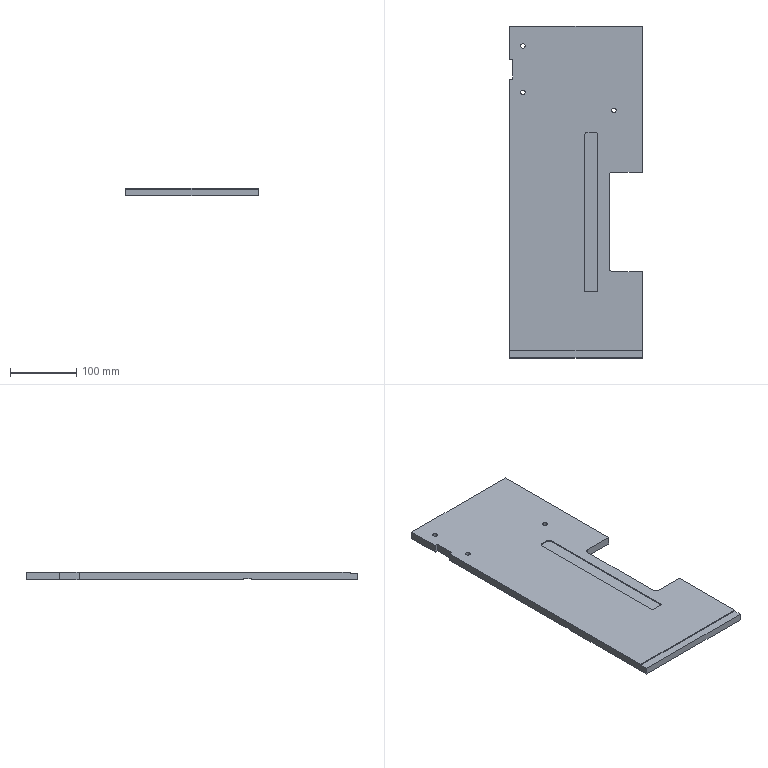Part | SolidWorks | features ICE 6, Fillet 2, Extrusion 1 | 1 solid | 35 faces | box 200 x 500 x 12 mm | volume 1093684 mm3 | plane 25 | cylinder 10 | commonest cylinder face diameters 7 x6 10 x4
STEP:
#1=CARTESIAN_POINT('',(-83.5,220.,-6.));
#2=VERTEX_POINT('',#1);
#3=CARTESIAN_POINT('',(-76.5,220.,-6.));
#4=VERTEX_POINT('',#3);
#5=CARTESIAN_POINT('',(-80.,220.,-6.));
#6=DIRECTION('',(0.,0.,1.));
#7=DIRECTION('',(-1.,0.,0.));
#8=AXIS2_PLACEMENT_3D('',#5,#6,#7);
#9=CIRCLE('',#8,3.5);
#10=EDGE_CURVE('',#2,#4,#9,.T.);
#11=ORIENTED_EDGE('',*,*,#10,.F.);
#12=CARTESIAN_POINT('',(-83.5,220.,6.));
#13=VERTEX_POINT('',#12);
#14=CARTESIAN_POINT('',(-83.5,220.,-6.001));
#15=DIRECTION('',(0.,0.,1.));
#16=VECTOR('',#15,1000.);
#17=LINE('',#14,#16);
#18=EDGE_CURVE('',#2,#13,#17,.T.);
#19=ORIENTED_EDGE('',*,*,#18,.T.);
#20=CARTESIAN_POINT('',(-76.5,220.,6.));
#21=VERTEX_POINT('',#20);
#22=CARTESIAN_POINT('',(-80.,220.,6.));
#23=DIRECTION('',(0.,0.,1.));
#24=DIRECTION('',(1.,0.,0.));
#25=AXIS2_PLACEMENT_3D('',#22,#23,#24);
#26=CIRCLE('',#25,3.5);
#27=EDGE_CURVE('',#13,#21,#26,.T.);
#28=ORIENTED_EDGE('',*,*,#27,.T.);
#29=CARTESIAN_POINT('',(-76.5,220.,-6.001));
#30=DIRECTION('',(0.,0.,1.));
#31=VECTOR('',#30,1000.);
#32=LINE('',#29,#31);
#33=EDGE_CURVE('',#4,#21,#32,.T.);
#34=ORIENTED_EDGE('',*,*,#33,.F.);
#35=EDGE_LOOP('',(#11,#19,#28,#34));
#36=FACE_OUTER_BOUND('',#35,.T.);
#37=CARTESIAN_POINT('',(-80.,220.,-6.001));
#38=DIRECTION('',(0.,0.,1.));
#39=DIRECTION('',(1.,0.,0.));
#40=AXIS2_PLACEMENT_3D('',#37,#38,#39);
#41=CYLINDRICAL_SURFACE('',#40,3.5);
#42=ADVANCED_FACE('',(#36),#41,.F.);
#43=CARTESIAN_POINT('',(-83.5,150.,-6.));
#44=VERTEX_POINT('',#43);
#45=CARTESIAN_POINT('',(-76.5,150.,-6.));
#46=VERTEX_POINT('',#45);
#47=CARTESIAN_POINT('',(-80.,150.,-6.));
#48=DIRECTION('',(0.,0.,1.));
#49=DIRECTION('',(-1.,0.,0.));
#50=AXIS2_PLACEMENT_3D('',#47,#48,#49);
#51=CIRCLE('',#50,3.5);
#52=EDGE_CURVE('',#44,#46,#51,.T.);
#53=ORIENTED_EDGE('',*,*,#52,.F.);
#54=CARTESIAN_POINT('',(-83.5,150.,6.));
#55=VERTEX_POINT('',#54);
#56=CARTESIAN_POINT('',(-83.5,150.,-6.001));
#57=DIRECTION('',(0.,0.,1.));
#58=VECTOR('',#57,1000.);
#59=LINE('',#56,#58);
#60=EDGE_CURVE('',#44,#55,#59,.T.);
#61=ORIENTED_EDGE('',*,*,#60,.T.);
#62=CARTESIAN_POINT('',(-76.5,150.,6.));
#63=VERTEX_POINT('',#62);
#64=CARTESIAN_POINT('',(-80.,150.,6.));
#65=DIRECTION('',(0.,0.,1.));
#66=DIRECTION('',(1.,0.,0.));
#67=AXIS2_PLACEMENT_3D('',#64,#65,#66);
#68=CIRCLE('',#67,3.5);
#69=EDGE_CURVE('',#55,#63,#68,.T.);
#70=ORIENTED_EDGE('',*,*,#69,.T.);
#71=CARTESIAN_POINT('',(-76.5,150.,-6.001));
#72=DIRECTION('',(0.,0.,1.));
#73=VECTOR('',#72,1000.);
#74=LINE('',#71,#73);
#75=EDGE_CURVE('',#46,#63,#74,.T.);
#76=ORIENTED_EDGE('',*,*,#75,.F.);
#77=EDGE_LOOP('',(#53,#61,#70,#76));
#78=FACE_OUTER_BOUND('',#77,.T.);
#79=CARTESIAN_POINT('',(-80.,150.,-6.001));
#80=DIRECTION('',(0.,0.,1.));
#81=DIRECTION('',(1.,0.,0.));
#82=AXIS2_PLACEMENT_3D('',#79,#80,#81);
#83=CYLINDRICAL_SURFACE('',#82,3.5);
#84=ADVANCED_FACE('',(#78),#83,.F.);
#85=CARTESIAN_POINT('',(53.5,123.,-6.));
#86=VERTEX_POINT('',#85);
#87=CARTESIAN_POINT('',(60.5,123.,-6.));
#88=VERTEX_POINT('',#87);
#89=CARTESIAN_POINT('',(57.,123.,-6.));
#90=DIRECTION('',(0.,0.,1.));
#91=DIRECTION('',(-1.,0.,0.));
#92=AXIS2_PLACEMENT_3D('',#89,#90,#91);
#93=CIRCLE('',#92,3.5);
#94=EDGE_CURVE('',#86,#88,#93,.T.);
#95=ORIENTED_EDGE('',*,*,#94,.F.);
#96=CARTESIAN_POINT('',(53.5,123.,6.));
#97=VERTEX_POINT('',#96);
#98=CARTESIAN_POINT('',(53.5,123.,-6.001));
#99=DIRECTION('',(0.,0.,1.));
#100=VECTOR('',#99,1000.);
#101=LINE('',#98,#100);
#102=EDGE_CURVE('',#86,#97,#101,.T.);
#103=ORIENTED_EDGE('',*,*,#102,.T.);
#104=CARTESIAN_POINT('',(60.5,123.,6.));
#105=VERTEX_POINT('',#104);
#106=CARTESIAN_POINT('',(57.,123.,6.));
#107=DIRECTION('',(0.,0.,1.));
#108=DIRECTION('',(1.,0.,0.));
#109=AXIS2_PLACEMENT_3D('',#106,#107,#108);
#110=CIRCLE('',#109,3.5);
#111=EDGE_CURVE('',#97,#105,#110,.T.);
#112=ORIENTED_EDGE('',*,*,#111,.T.);
#113=CARTESIAN_POINT('',(60.5,123.,-6.001));
#114=DIRECTION('',(0.,0.,1.));
#115=VECTOR('',#114,1000.);
#116=LINE('',#113,#115);
#117=EDGE_CURVE('',#88,#105,#116,.T.);
#118=ORIENTED_EDGE('',*,*,#117,.F.);
#119=EDGE_LOOP('',(#95,#103,#112,#118));
#120=FACE_OUTER_BOUND('',#119,.T.);
#121=CARTESIAN_POINT('',(57.,123.,-6.001));
#122=DIRECTION('',(0.,0.,1.));
#123=DIRECTION('',(1.,0.,0.));
#124=AXIS2_PLACEMENT_3D('',#121,#122,#123);
#125=CYLINDRICAL_SURFACE('',#124,3.5);
#126=ADVANCED_FACE('',(#120),#125,.F.);
#127=CARTESIAN_POINT('',(100.,30.,6.));
#128=VERTEX_POINT('',#127);
#129=CARTESIAN_POINT('',(100.,250.,6.));
#130=VERTEX_POINT('',#129);
#131=CARTESIAN_POINT('',(100.,-250.,6.));
#132=DIRECTION('',(0.,1.,0.));
#133=VECTOR('',#132,1000.);
#134=LINE('',#131,#133);
#135=EDGE_CURVE('',#128,#130,#134,.T.);
#136=ORIENTED_EDGE('',*,*,#135,.F.);
#137=CARTESIAN_POINT('',(100.,30.,-6.));
#138=VERTEX_POINT('',#137);
#139=CARTESIAN_POINT('',(100.,30.,6.001));
#140=DIRECTION('',(0.,0.,-1.));
#141=VECTOR('',#140,1000.);
#142=LINE('',#139,#141);
#143=EDGE_CURVE('',#128,#138,#142,.T.);
#144=ORIENTED_EDGE('',*,*,#143,.T.);
#145=CARTESIAN_POINT('',(100.,250.,-6.));
#146=VERTEX_POINT('',#145);
#147=CARTESIAN_POINT('',(100.,-250.,-6.));
#148=DIRECTION('',(0.,1.,0.));
#149=VECTOR('',#148,1000.);
#150=LINE('',#147,#149);
#151=EDGE_CURVE('',#138,#146,#150,.T.);
#152=ORIENTED_EDGE('',*,*,#151,.T.);
#153=CARTESIAN_POINT('',(100.,250.,6.));
#154=DIRECTION('',(0.,0.,-1.));
#155=VECTOR('',#154,1000.);
#156=LINE('',#153,#155);
#157=EDGE_CURVE('',#130,#146,#156,.T.);
#158=ORIENTED_EDGE('',*,*,#157,.F.);
#159=EDGE_LOOP('',(#136,#144,#152,#158));
#160=FACE_OUTER_BOUND('',#159,.T.);
#161=CARTESIAN_POINT('',(100.,-250.,6.));
#162=DIRECTION('',(-1.,0.,0.));
#163=DIRECTION('',(0.,0.,1.));
#164=AXIS2_PLACEMENT_3D('',#161,#162,#163);
#165=PLANE('',#164);
#166=ADVANCED_FACE('',(#160),#165,.F.);
#167=CARTESIAN_POINT('',(-100.,170.,6.));
#168=VERTEX_POINT('',#167);
#169=CARTESIAN_POINT('',(-100.,-238.,6.));
#170=VERTEX_POINT('',#169);
#171=CARTESIAN_POINT('',(-100.,-250.,6.));
#172=DIRECTION('',(0.,-1.,0.));
#173=VECTOR('',#172,1000.);
#174=LINE('',#171,#173);
#175=EDGE_CURVE('',#168,#170,#174,.T.);
#176=ORIENTED_EDGE('',*,*,#175,.T.);
#177=CARTESIAN_POINT('',(100.,-238.,6.));
#178=VERTEX_POINT('',#177);
#179=CARTESIAN_POINT('',(-100.,-238.,6.));
#180=DIRECTION('',(-1.,0.,0.));
#181=VECTOR('',#180,1000.);
#182=LINE('',#179,#181);
#183=EDGE_CURVE('',#178,#170,#182,.T.);
#184=ORIENTED_EDGE('',*,*,#183,.F.);
#185=CARTESIAN_POINT('',(100.,-120.,6.));
#186=VERTEX_POINT('',#185);
#187=CARTESIAN_POINT('',(100.,-250.,6.));
#188=DIRECTION('',(0.,1.,0.));
#189=VECTOR('',#188,1000.);
#190=LINE('',#187,#189);
#191=EDGE_CURVE('',#178,#186,#190,.T.);
#192=ORIENTED_EDGE('',*,*,#191,.T.);
#193=CARTESIAN_POINT('',(55.,-120.,6.));
#194=VERTEX_POINT('',#193);
#195=CARTESIAN_POINT('',(100.,-120.,6.));
#196=DIRECTION('',(1.,0.,0.));
#197=VECTOR('',#196,1000.);
#198=LINE('',#195,#197);
#199=EDGE_CURVE('',#194,#186,#198,.T.);
#200=ORIENTED_EDGE('',*,*,#199,.F.);
#201=CARTESIAN_POINT('',(50.,-115.,6.));
#202=VERTEX_POINT('',#201);
#203=CARTESIAN_POINT('',(55.,-115.,6.));
#204=DIRECTION('',(0.,0.,-1.));
#205=DIRECTION('',(-1.,0.,0.));
#206=AXIS2_PLACEMENT_3D('',#203,#204,#205);
#207=CIRCLE('',#206,5.);
#208=EDGE_CURVE('',#194,#202,#207,.T.);
#209=ORIENTED_EDGE('',*,*,#208,.T.);
#210=CARTESIAN_POINT('',(50.,25.,6.));
#211=VERTEX_POINT('',#210);
#212=CARTESIAN_POINT('',(50.,-120.,6.));
#213=DIRECTION('',(0.,-1.,0.));
#214=VECTOR('',#213,1000.);
#215=LINE('',#212,#214);
#216=EDGE_CURVE('',#211,#202,#215,.T.);
#217=ORIENTED_EDGE('',*,*,#216,.F.);
#218=CARTESIAN_POINT('',(55.,30.,6.));
#219=VERTEX_POINT('',#218);
#220=CARTESIAN_POINT('',(55.,25.,6.));
#221=DIRECTION('',(0.,0.,-1.));
#222=DIRECTION('',(-1.,0.,0.));
#223=AXIS2_PLACEMENT_3D('',#220,#221,#222);
#224=CIRCLE('',#223,5.);
#225=EDGE_CURVE('',#211,#219,#224,.T.);
#226=ORIENTED_EDGE('',*,*,#225,.T.);
#227=CARTESIAN_POINT('',(100.,30.,6.));
#228=DIRECTION('',(-1.,0.,0.));
#229=VECTOR('',#228,1000.);
#230=LINE('',#227,#229);
#231=EDGE_CURVE('',#128,#219,#230,.T.);
#232=ORIENTED_EDGE('',*,*,#231,.F.);
#233=ORIENTED_EDGE('',*,*,#135,.T.);
#234=CARTESIAN_POINT('',(-100.,250.,6.));
#235=VERTEX_POINT('',#234);
#236=CARTESIAN_POINT('',(-100.,250.,6.));
#237=DIRECTION('',(-1.,0.,0.));
#238=VECTOR('',#237,1000.);
#239=LINE('',#236,#238);
#240=EDGE_CURVE('',#130,#235,#239,.T.);
#241=ORIENTED_EDGE('',*,*,#240,.T.);
#242=CARTESIAN_POINT('',(-100.,200.,6.));
#243=VERTEX_POINT('',#242);
#244=CARTESIAN_POINT('',(-100.,-250.,6.));
#245=DIRECTION('',(0.,-1.,0.));
#246=VECTOR('',#245,1000.);
#247=LINE('',#244,#246);
#248=EDGE_CURVE('',#235,#243,#247,.T.);
#249=ORIENTED_EDGE('',*,*,#248,.T.);
#250=CARTESIAN_POINT('',(-95.,200.,6.));
#251=VERTEX_POINT('',#250);
#252=CARTESIAN_POINT('',(-95.,200.,6.));
#253=DIRECTION('',(-1.,0.,0.));
#254=VECTOR('',#253,1000.);
#255=LINE('',#252,#254);
#256=EDGE_CURVE('',#251,#243,#255,.T.);
#257=ORIENTED_EDGE('',*,*,#256,.F.);
#258=CARTESIAN_POINT('',(-95.,170.,6.));
#259=VERTEX_POINT('',#258);
#260=CARTESIAN_POINT('',(-95.,170.,6.));
#261=DIRECTION('',(0.,1.,0.));
#262=VECTOR('',#261,1000.);
#263=LINE('',#260,#262);
#264=EDGE_CURVE('',#259,#251,#263,.T.);
#265=ORIENTED_EDGE('',*,*,#264,.F.);
#266=CARTESIAN_POINT('',(-100.,170.,6.));
#267=DIRECTION('',(1.,0.,0.));
#268=VECTOR('',#267,1000.);
#269=LINE('',#266,#268);
#270=EDGE_CURVE('',#168,#259,#269,.T.);
#271=ORIENTED_EDGE('',*,*,#270,.F.);
#272=EDGE_LOOP('',(#176,#184,#192,#200,#209,#217,#226,#232,#233,#241,#249,#257,#265,#271));
#273=FACE_OUTER_BOUND('',#272,.T.);
#274=CARTESIAN_POINT('',(57.,123.,6.));
#275=DIRECTION('',(0.,0.,1.));
#276=DIRECTION('',(1.,0.,0.));
#277=AXIS2_PLACEMENT_3D('',#274,#275,#276);
#278=CIRCLE('',#277,3.5);
#279=EDGE_CURVE('',#105,#97,#278,.T.);
#280=ORIENTED_EDGE('',*,*,#279,.F.);
#281=ORIENTED_EDGE('',*,*,#111,.F.);
#282=EDGE_LOOP('',(#280,#281));
#283=FACE_BOUND('',#282,.T.);
#284=CARTESIAN_POINT('',(-80.,150.,6.));
#285=DIRECTION('',(0.,0.,1.));
#286=DIRECTION('',(1.,0.,0.));
#287=AXIS2_PLACEMENT_3D('',#284,#285,#286);
#288=CIRCLE('',#287,3.5);
#289=EDGE_CURVE('',#63,#55,#288,.T.);
#290=ORIENTED_EDGE('',*,*,#289,.F.);
#291=ORIENTED_EDGE('',*,*,#69,.F.);
#292=EDGE_LOOP('',(#290,#291));
#293=FACE_BOUND('',#292,.T.);
#294=CARTESIAN_POINT('',(-80.,220.,6.));
#295=DIRECTION('',(0.,0.,1.));
#296=DIRECTION('',(1.,0.,0.));
#297=AXIS2_PLACEMENT_3D('',#294,#295,#296);
#298=CIRCLE('',#297,3.5);
#299=EDGE_CURVE('',#21,#13,#298,.T.);
#300=ORIENTED_EDGE('',*,*,#299,.F.);
#301=ORIENTED_EDGE('',*,*,#27,.F.);
#302=EDGE_LOOP('',(#300,#301));
#303=FACE_BOUND('',#302,.T.);
#304=CARTESIAN_POINT('',(18.,90.,6.));
#305=VERTEX_POINT('',#304);
#306=CARTESIAN_POINT('',(28.,90.,6.));
#307=VERTEX_POINT('',#306);
#308=CARTESIAN_POINT('',(33.,90.,6.));
#309=DIRECTION('',(1.,0.,0.));
#310=VECTOR('',#309,1000.);
#311=LINE('',#308,#310);
#312=EDGE_CURVE('',#305,#307,#311,.T.);
#313=ORIENTED_EDGE('',*,*,#312,.T.);
#314=CARTESIAN_POINT('',(33.,85.,6.));
#315=VERTEX_POINT('',#314);
#316=CARTESIAN_POINT('',(28.,85.,6.));
#317=DIRECTION('',(0.,0.,-1.));
#318=DIRECTION('',(-1.,0.,0.));
#319=AXIS2_PLACEMENT_3D('',#316,#317,#318);
#320=CIRCLE('',#319,5.);
#321=EDGE_CURVE('',#307,#315,#320,.T.);
#322=ORIENTED_EDGE('',*,*,#321,.T.);
#323=CARTESIAN_POINT('',(33.,-150.,6.));
#324=VERTEX_POINT('',#323);
#325=CARTESIAN_POINT('',(33.,-150.,6.));
#326=DIRECTION('',(0.,-1.,0.));
#327=VECTOR('',#326,1000.);
#328=LINE('',#325,#327);
#329=EDGE_CURVE('',#315,#324,#328,.T.);
#330=ORIENTED_EDGE('',*,*,#329,.T.);
#331=CARTESIAN_POINT('',(13.,-150.,6.));
#332=VERTEX_POINT('',#331);
#333=CARTESIAN_POINT('',(33.,-150.,6.));
#334=DIRECTION('',(-1.,0.,0.));
#335=VECTOR('',#334,1000.);
#336=LINE('',#333,#335);
#337=EDGE_CURVE('',#324,#332,#336,.T.);
#338=ORIENTED_EDGE('',*,*,#337,.T.);
#339=CARTESIAN_POINT('',(13.,85.,6.));
#340=VERTEX_POINT('',#339);
#341=CARTESIAN_POINT('',(13.,-150.,6.));
#342=DIRECTION('',(0.,1.,0.));
#343=VECTOR('',#342,1000.);
#344=LINE('',#341,#343);
#345=EDGE_CURVE('',#332,#340,#344,.T.);
#346=ORIENTED_EDGE('',*,*,#345,.T.);
#347=CARTESIAN_POINT('',(18.,85.,6.));
#348=DIRECTION('',(0.,0.,-1.));
#349=DIRECTION('',(-1.,0.,0.));
#350=AXIS2_PLACEMENT_3D('',#347,#348,#349);
#351=CIRCLE('',#350,5.);
#352=EDGE_CURVE('',#340,#305,#351,.T.);
#353=ORIENTED_EDGE('',*,*,#352,.T.);
#354=EDGE_LOOP('',(#313,#322,#330,#338,#346,#353));
#355=FACE_BOUND('',#354,.T.);
#356=CARTESIAN_POINT('',(0.,0.,6.));
#357=DIRECTION('',(0.,0.,-1.));
#358=DIRECTION('',(-1.,0.,0.));
#359=AXIS2_PLACEMENT_3D('',#356,#357,#358);
#360=PLANE('',#359);
#361=ADVANCED_FACE('',(#273,#283,#293,#303,#355),#360,.F.);
#362=CARTESIAN_POINT('',(-100.,-238.,4.5));
#363=VERTEX_POINT('',#362);
#364=CARTESIAN_POINT('',(-100.,-250.,4.5));
#365=VERTEX_POINT('',#364);
#366=CARTESIAN_POINT('',(-100.,-250.,4.5));
#367=DIRECTION('',(0.,-1.,0.));
#368=VECTOR('',#367,1000.);
#369=LINE('',#366,#368);
#370=EDGE_CURVE('',#363,#365,#369,.T.);
#371=ORIENTED_EDGE('',*,*,#370,.F.);
#372=CARTESIAN_POINT('',(-100.,-238.,4.5));
#373=DIRECTION('',(0.,0.,1.));
#374=VECTOR('',#373,1000.);
#375=LINE('',#372,#374);
#376=EDGE_CURVE('',#363,#170,#375,.T.);
#377=ORIENTED_EDGE('',*,*,#376,.T.);
#378=ORIENTED_EDGE('',*,*,#175,.F.);
#379=CARTESIAN_POINT('',(-100.,170.,-6.));
#380=VERTEX_POINT('',#379);
#381=CARTESIAN_POINT('',(-100.,170.,-6.001));
#382=DIRECTION('',(0.,0.,1.));
#383=VECTOR('',#382,1000.);
#384=LINE('',#381,#383);
#385=EDGE_CURVE('',#380,#168,#384,.T.);
#386=ORIENTED_EDGE('',*,*,#385,.F.);
#387=CARTESIAN_POINT('',(-100.,-78.,-6.));
#388=VERTEX_POINT('',#387);
#389=CARTESIAN_POINT('',(-100.,-250.,-6.));
#390=DIRECTION('',(0.,-1.,0.));
#391=VECTOR('',#390,1000.);
#392=LINE('',#389,#391);
#393=EDGE_CURVE('',#380,#388,#392,.T.);
#394=ORIENTED_EDGE('',*,*,#393,.T.);
#395=CARTESIAN_POINT('',(-100.,-78.,-4.5));
#396=VERTEX_POINT('',#395);
#397=CARTESIAN_POINT('',(-100.,-78.,-4.5));
#398=DIRECTION('',(0.,0.,-1.));
#399=VECTOR('',#398,1000.);
#400=LINE('',#397,#399);
#401=EDGE_CURVE('',#396,#388,#400,.T.);
#402=ORIENTED_EDGE('',*,*,#401,.F.);
#403=CARTESIAN_POINT('',(-100.,-89.,-4.5));
#404=VERTEX_POINT('',#403);
#405=CARTESIAN_POINT('',(-100.,-89.,-4.5));
#406=DIRECTION('',(0.,-1.,0.));
#407=VECTOR('',#406,1000.);
#408=LINE('',#405,#407);
#409=EDGE_CURVE('',#396,#404,#408,.T.);
#410=ORIENTED_EDGE('',*,*,#409,.T.);
#411=CARTESIAN_POINT('',(-100.,-89.,-6.));
#412=VERTEX_POINT('',#411);
#413=CARTESIAN_POINT('',(-100.,-89.,-4.5));
#414=DIRECTION('',(0.,0.,-1.));
#415=VECTOR('',#414,1000.);
#416=LINE('',#413,#415);
#417=EDGE_CURVE('',#404,#412,#416,.T.);
#418=ORIENTED_EDGE('',*,*,#417,.T.);
#419=CARTESIAN_POINT('',(-100.,-250.,-6.));
#420=VERTEX_POINT('',#419);
#421=CARTESIAN_POINT('',(-100.,-250.,-6.));
#422=DIRECTION('',(0.,-1.,0.));
#423=VECTOR('',#422,1000.);
#424=LINE('',#421,#423);
#425=EDGE_CURVE('',#412,#420,#424,.T.);
#426=ORIENTED_EDGE('',*,*,#425,.T.);
#427=CARTESIAN_POINT('',(-100.,-250.,6.));
#428=DIRECTION('',(0.,0.,-1.));
#429=VECTOR('',#428,1000.);
#430=LINE('',#427,#429);
#431=EDGE_CURVE('',#365,#420,#430,.T.);
#432=ORIENTED_EDGE('',*,*,#431,.F.);
#433=EDGE_LOOP('',(#371,#377,#378,#386,#394,#402,#410,#418,#426,#432));
#434=FACE_OUTER_BOUND('',#433,.T.);
#435=CARTESIAN_POINT('',(-100.,-250.,6.));
#436=DIRECTION('',(1.,0.,0.));
#437=DIRECTION('',(0.,0.,-1.));
#438=AXIS2_PLACEMENT_3D('',#435,#436,#437);
#439=PLANE('',#438);
#440=ADVANCED_FACE('',(#434),#439,.F.);
#441=ORIENTED_EDGE('',*,*,#191,.F.);
#442=CARTESIAN_POINT('',(100.,-238.,4.5));
#443=VERTEX_POINT('',#442);
#444=CARTESIAN_POINT('',(100.,-238.,4.5));
#445=DIRECTION('',(0.,0.,1.));
#446=VECTOR('',#445,1000.);
#447=LINE('',#444,#446);
#448=EDGE_CURVE('',#443,#178,#447,.T.);
#449=ORIENTED_EDGE('',*,*,#448,.F.);
#450=CARTESIAN_POINT('',(100.,-250.,4.5));
#451=VERTEX_POINT('',#450);
#452=CARTESIAN_POINT('',(100.,-250.,4.5));
#453=DIRECTION('',(0.,1.,0.));
#454=VECTOR('',#453,1000.);
#455=LINE('',#452,#454);
#456=EDGE_CURVE('',#451,#443,#455,.T.);
#457=ORIENTED_EDGE('',*,*,#456,.F.);
#458=CARTESIAN_POINT('',(100.,-250.,-6.));
#459=VERTEX_POINT('',#458);
#460=CARTESIAN_POINT('',(100.,-250.,6.));
#461=DIRECTION('',(0.,0.,-1.));
#462=VECTOR('',#461,1000.);
#463=LINE('',#460,#462);
#464=EDGE_CURVE('',#451,#459,#463,.T.);
#465=ORIENTED_EDGE('',*,*,#464,.T.);
#466=CARTESIAN_POINT('',(100.,-120.,-6.));
#467=VERTEX_POINT('',#466);
#468=CARTESIAN_POINT('',(100.,-250.,-6.));
#469=DIRECTION('',(0.,1.,0.));
#470=VECTOR('',#469,1000.);
#471=LINE('',#468,#470);
#472=EDGE_CURVE('',#459,#467,#471,.T.);
#473=ORIENTED_EDGE('',*,*,#472,.T.);
#474=CARTESIAN_POINT('',(100.,-120.,6.001));
#475=DIRECTION('',(0.,0.,-1.));
#476=VECTOR('',#475,1000.);
#477=LINE('',#474,#476);
#478=EDGE_CURVE('',#186,#467,#477,.T.);
#479=ORIENTED_EDGE('',*,*,#478,.F.);
#480=EDGE_LOOP('',(#441,#449,#457,#465,#473,#479));
#481=FACE_OUTER_BOUND('',#480,.T.);
#482=CARTESIAN_POINT('',(100.,-250.,6.));
#483=DIRECTION('',(-1.,0.,0.));
#484=DIRECTION('',(0.,0.,1.));
#485=AXIS2_PLACEMENT_3D('',#482,#483,#484);
#486=PLANE('',#485);
#487=ADVANCED_FACE('',(#481),#486,.F.);
#488=CARTESIAN_POINT('',(-100.,250.,-6.));
#489=VERTEX_POINT('',#488);
#490=CARTESIAN_POINT('',(-100.,200.,-6.));
#491=VERTEX_POINT('',#490);
#492=CARTESIAN_POINT('',(-100.,-250.,-6.));
#493=DIRECTION('',(0.,-1.,0.));
#494=VECTOR('',#493,1000.);
#495=LINE('',#492,#494);
#496=EDGE_CURVE('',#489,#491,#495,.T.);
#497=ORIENTED_EDGE('',*,*,#496,.T.);
#498=CARTESIAN_POINT('',(-100.,200.,-6.001));
#499=DIRECTION('',(0.,0.,1.));
#500=VECTOR('',#499,1000.);
#501=LINE('',#498,#500);
#502=EDGE_CURVE('',#491,#243,#501,.T.);
#503=ORIENTED_EDGE('',*,*,#502,.T.);
#504=ORIENTED_EDGE('',*,*,#248,.F.);
#505=CARTESIAN_POINT('',(-100.,250.,6.));
#506=DIRECTION('',(0.,0.,-1.));
#507=VECTOR('',#506,1000.);
#508=LINE('',#505,#507);
#509=EDGE_CURVE('',#235,#489,#508,.T.);
#510=ORIENTED_EDGE('',*,*,#509,.T.);
#511=EDGE_LOOP('',(#497,#503,#504,#510));
#512=FACE_OUTER_BOUND('',#511,.T.);
#513=CARTESIAN_POINT('',(-100.,-250.,6.));
#514=DIRECTION('',(1.,0.,0.));
#515=DIRECTION('',(0.,0.,-1.));
#516=AXIS2_PLACEMENT_3D('',#513,#514,#515);
#517=PLANE('',#516);
#518=ADVANCED_FACE('',(#512),#517,.F.);
#519=CARTESIAN_POINT('',(50.,-115.,-6.));
#520=VERTEX_POINT('',#519);
#521=CARTESIAN_POINT('',(50.,-89.,-6.));
#522=VERTEX_POINT('',#521);
#523=CARTESIAN_POINT('',(50.,-120.,-6.));
#524=DIRECTION('',(0.,1.,0.));
#525=VECTOR('',#524,1000.);
#526=LINE('',#523,#525);
#527=EDGE_CURVE('',#520,#522,#526,.T.);
#528=ORIENTED_EDGE('',*,*,#527,.F.);
#529=CARTESIAN_POINT('',(55.,-120.,-6.));
#530=VERTEX_POINT('',#529);
#531=CARTESIAN_POINT('',(55.,-115.,-6.));
#532=DIRECTION('',(0.,0.,1.));
#533=DIRECTION('',(-1.,0.,0.));
#534=AXIS2_PLACEMENT_3D('',#531,#532,#533);
#535=CIRCLE('',#534,5.);
#536=EDGE_CURVE('',#520,#530,#535,.T.);
#537=ORIENTED_EDGE('',*,*,#536,.T.);
#538=CARTESIAN_POINT('',(100.,-120.,-6.));
#539=DIRECTION('',(-1.,0.,0.));
#540=VECTOR('',#539,1000.);
#541=LINE('',#538,#540);
#542=EDGE_CURVE('',#467,#530,#541,.T.);
#543=ORIENTED_EDGE('',*,*,#542,.F.);
#544=ORIENTED_EDGE('',*,*,#472,.F.);
#545=CARTESIAN_POINT('',(-100.,-250.,-6.));
#546=DIRECTION('',(1.,0.,0.));
#547=VECTOR('',#546,1000.);
#548=LINE('',#545,#547);
#549=EDGE_CURVE('',#420,#459,#548,.T.);
#550=ORIENTED_EDGE('',*,*,#549,.F.);
#551=ORIENTED_EDGE('',*,*,#425,.F.);
#552=CARTESIAN_POINT('',(-100.,-89.,-6.));
#553=DIRECTION('',(1.,0.,0.));
#554=VECTOR('',#553,1000.);
#555=LINE('',#552,#554);
#556=EDGE_CURVE('',#412,#522,#555,.T.);
#557=ORIENTED_EDGE('',*,*,#556,.T.);
#558=EDGE_LOOP('',(#528,#537,#543,#544,#550,#551,#557));
#559=FACE_OUTER_BOUND('',#558,.T.);
#560=CARTESIAN_POINT('',(0.,0.,-6.));
#561=DIRECTION('',(0.,0.,-1.));
#562=DIRECTION('',(-1.,0.,0.));
#563=AXIS2_PLACEMENT_3D('',#560,#561,#562);
#564=PLANE('',#563);
#565=ADVANCED_FACE('',(#559),#564,.T.);
#566=CARTESIAN_POINT('',(55.,30.,-6.));
#567=VERTEX_POINT('',#566);
#568=CARTESIAN_POINT('',(100.,30.,-6.));
#569=DIRECTION('',(1.,0.,0.));
#570=VECTOR('',#569,1000.);
#571=LINE('',#568,#570);
#572=EDGE_CURVE('',#567,#138,#571,.T.);
#573=ORIENTED_EDGE('',*,*,#572,.F.);
#574=CARTESIAN_POINT('',(50.,25.,-6.));
#575=VERTEX_POINT('',#574);
#576=CARTESIAN_POINT('',(55.,25.,-6.));
#577=DIRECTION('',(0.,0.,1.));
#578=DIRECTION('',(-1.,0.,0.));
#579=AXIS2_PLACEMENT_3D('',#576,#577,#578);
#580=CIRCLE('',#579,5.);
#581=EDGE_CURVE('',#567,#575,#580,.T.);
#582=ORIENTED_EDGE('',*,*,#581,.T.);
#583=CARTESIAN_POINT('',(50.,-78.,-6.));
#584=VERTEX_POINT('',#583);
#585=CARTESIAN_POINT('',(50.,-120.,-6.));
#586=DIRECTION('',(0.,1.,0.));
#587=VECTOR('',#586,1000.);
#588=LINE('',#585,#587);
#589=EDGE_CURVE('',#584,#575,#588,.T.);
#590=ORIENTED_EDGE('',*,*,#589,.F.);
#591=CARTESIAN_POINT('',(-100.,-78.,-6.));
#592=DIRECTION('',(-1.,0.,0.));
#593=VECTOR('',#592,1000.);
#594=LINE('',#591,#593);
#595=EDGE_CURVE('',#584,#388,#594,.T.);
#596=ORIENTED_EDGE('',*,*,#595,.T.);
#597=ORIENTED_EDGE('',*,*,#393,.F.);
#598=CARTESIAN_POINT('',(-95.,170.,-6.));
#599=VERTEX_POINT('',#598);
#600=CARTESIAN_POINT('',(-100.,170.,-6.));
#601=DIRECTION('',(1.,0.,0.));
#602=VECTOR('',#601,1000.);
#603=LINE('',#600,#602);
#604=EDGE_CURVE('',#380,#599,#603,.T.);
#605=ORIENTED_EDGE('',*,*,#604,.T.);
#606=CARTESIAN_POINT('',(-95.,200.,-6.));
#607=VERTEX_POINT('',#606);
#608=CARTESIAN_POINT('',(-95.,170.,-6.));
#609=DIRECTION('',(0.,1.,0.));
#610=VECTOR('',#609,1000.);
#611=LINE('',#608,#610);
#612=EDGE_CURVE('',#599,#607,#611,.T.);
#613=ORIENTED_EDGE('',*,*,#612,.T.);
#614=CARTESIAN_POINT('',(-95.,200.,-6.));
#615=DIRECTION('',(-1.,0.,0.));
#616=VECTOR('',#615,1000.);
#617=LINE('',#614,#616);
#618=EDGE_CURVE('',#607,#491,#617,.T.);
#619=ORIENTED_EDGE('',*,*,#618,.T.);
#620=ORIENTED_EDGE('',*,*,#496,.F.);
#621=CARTESIAN_POINT('',(-100.,250.,-6.));
#622=DIRECTION('',(-1.,0.,0.));
#623=VECTOR('',#622,1000.);
#624=LINE('',#621,#623);
#625=EDGE_CURVE('',#146,#489,#624,.T.);
#626=ORIENTED_EDGE('',*,*,#625,.F.);
#627=ORIENTED_EDGE('',*,*,#151,.F.);
#628=EDGE_LOOP('',(#573,#582,#590,#596,#597,#605,#613,#619,#620,#626,#627));
#629=FACE_OUTER_BOUND('',#628,.T.);
#630=CARTESIAN_POINT('',(-80.,220.,-6.));
#631=DIRECTION('',(0.,0.,1.));
#632=DIRECTION('',(-1.,0.,0.));
#633=AXIS2_PLACEMENT_3D('',#630,#631,#632);
#634=CIRCLE('',#633,3.5);
#635=EDGE_CURVE('',#4,#2,#634,.T.);
#636=ORIENTED_EDGE('',*,*,#635,.T.);
#637=ORIENTED_EDGE('',*,*,#10,.T.);
#638=EDGE_LOOP('',(#636,#637));
#639=FACE_BOUND('',#638,.T.);
#640=CARTESIAN_POINT('',(-80.,150.,-6.));
#641=DIRECTION('',(0.,0.,1.));
#642=DIRECTION('',(-1.,0.,0.));
#643=AXIS2_PLACEMENT_3D('',#640,#641,#642);
#644=CIRCLE('',#643,3.5);
#645=EDGE_CURVE('',#46,#44,#644,.T.);
#646=ORIENTED_EDGE('',*,*,#645,.T.);
#647=ORIENTED_EDGE('',*,*,#52,.T.);
#648=EDGE_LOOP('',(#646,#647));
#649=FACE_BOUND('',#648,.T.);
#650=CARTESIAN_POINT('',(57.,123.,-6.));
#651=DIRECTION('',(0.,0.,1.));
#652=DIRECTION('',(-1.,0.,0.));
#653=AXIS2_PLACEMENT_3D('',#650,#651,#652);
#654=CIRCLE('',#653,3.5);
#655=EDGE_CURVE('',#88,#86,#654,.T.);
#656=ORIENTED_EDGE('',*,*,#655,.T.);
#657=ORIENTED_EDGE('',*,*,#94,.T.);
#658=EDGE_LOOP('',(#656,#657));
#659=FACE_BOUND('',#658,.T.);
#660=CARTESIAN_POINT('',(0.,0.,-6.));
#661=DIRECTION('',(0.,0.,-1.));
#662=DIRECTION('',(-1.,0.,0.));
#663=AXIS2_PLACEMENT_3D('',#660,#661,#662);
#664=PLANE('',#663);
#665=ADVANCED_FACE('',(#629,#639,#649,#659),#664,.T.);
#666=ORIENTED_EDGE('',*,*,#625,.T.);
#667=ORIENTED_EDGE('',*,*,#509,.F.);
#668=ORIENTED_EDGE('',*,*,#240,.F.);
#669=ORIENTED_EDGE('',*,*,#157,.T.);
#670=EDGE_LOOP('',(#666,#667,#668,#669));
#671=FACE_OUTER_BOUND('',#670,.T.);
#672=CARTESIAN_POINT('',(-100.,250.,6.));
#673=DIRECTION('',(0.,-1.,0.));
#674=DIRECTION('',(0.,0.,-1.));
#675=AXIS2_PLACEMENT_3D('',#672,#673,#674);
#676=PLANE('',#675);
#677=ADVANCED_FACE('',(#671),#676,.F.);
#678=ORIENTED_EDGE('',*,*,#464,.F.);
#679=CARTESIAN_POINT('',(-100.,-250.,4.5));
#680=DIRECTION('',(1.,0.,0.));
#681=VECTOR('',#680,1000.);
#682=LINE('',#679,#681);
#683=EDGE_CURVE('',#365,#451,#682,.T.);
#684=ORIENTED_EDGE('',*,*,#683,.F.);
#685=ORIENTED_EDGE('',*,*,#431,.T.);
#686=ORIENTED_EDGE('',*,*,#549,.T.);
#687=EDGE_LOOP('',(#678,#684,#685,#686));
#688=FACE_OUTER_BOUND('',#687,.T.);
#689=CARTESIAN_POINT('',(-100.,-250.,6.));
#690=DIRECTION('',(0.,1.,0.));
#691=DIRECTION('',(0.,0.,1.));
#692=AXIS2_PLACEMENT_3D('',#689,#690,#691);
#693=PLANE('',#692);
#694=ADVANCED_FACE('',(#688),#693,.F.);
#695=CARTESIAN_POINT('',(50.,-89.,-4.5));
#696=VERTEX_POINT('',#695);
#697=CARTESIAN_POINT('',(50.,-89.,6.001));
#698=DIRECTION('',(0.,0.,-1.));
#699=VECTOR('',#698,1000.);
#700=LINE('',#697,#699);
#701=EDGE_CURVE('',#696,#522,#700,.T.);
#702=ORIENTED_EDGE('',*,*,#701,.T.);
#703=ORIENTED_EDGE('',*,*,#556,.F.);
#704=ORIENTED_EDGE('',*,*,#417,.F.);
#705=CARTESIAN_POINT('',(-100.,-89.,-4.5));
#706=DIRECTION('',(1.,0.,0.));
#707=VECTOR('',#706,1000.);
#708=LINE('',#705,#707);
#709=EDGE_CURVE('',#404,#696,#708,.T.);
#710=ORIENTED_EDGE('',*,*,#709,.T.);
#711=EDGE_LOOP('',(#702,#703,#704,#710));
#712=FACE_OUTER_BOUND('',#711,.T.);
#713=CARTESIAN_POINT('',(-100.,-89.,-4.5));
#714=DIRECTION('',(0.,1.,0.));
#715=DIRECTION('',(0.,0.,1.));
#716=AXIS2_PLACEMENT_3D('',#713,#714,#715);
#717=PLANE('',#716);
#718=ADVANCED_FACE('',(#712),#717,.T.);
#719=CARTESIAN_POINT('',(50.,-78.,-4.5));
#720=VERTEX_POINT('',#719);
#721=CARTESIAN_POINT('',(50.,-78.,6.001));
#722=DIRECTION('',(0.,0.,1.));
#723=VECTOR('',#722,1000.);
#724=LINE('',#721,#723);
#725=EDGE_CURVE('',#584,#720,#724,.T.);
#726=ORIENTED_EDGE('',*,*,#725,.T.);
#727=CARTESIAN_POINT('',(-100.,-78.,-4.5));
#728=DIRECTION('',(-1.,0.,0.));
#729=VECTOR('',#728,1000.);
#730=LINE('',#727,#729);
#731=EDGE_CURVE('',#720,#396,#730,.T.);
#732=ORIENTED_EDGE('',*,*,#731,.T.);
#733=ORIENTED_EDGE('',*,*,#401,.T.);
#734=ORIENTED_EDGE('',*,*,#595,.F.);
#735=EDGE_LOOP('',(#726,#732,#733,#734));
#736=FACE_OUTER_BOUND('',#735,.T.);
#737=CARTESIAN_POINT('',(-100.,-78.,-4.5));
#738=DIRECTION('',(0.,-1.,0.));
#739=DIRECTION('',(0.,0.,-1.));
#740=AXIS2_PLACEMENT_3D('',#737,#738,#739);
#741=PLANE('',#740);
#742=ADVANCED_FACE('',(#736),#741,.T.);
#743=CARTESIAN_POINT('',(50.,-120.,-4.5));
#744=DIRECTION('',(0.,-1.,0.));
#745=VECTOR('',#744,1000.);
#746=LINE('',#743,#745);
#747=EDGE_CURVE('',#720,#696,#746,.T.);
#748=ORIENTED_EDGE('',*,*,#747,.T.);
#749=ORIENTED_EDGE('',*,*,#709,.F.);
#750=ORIENTED_EDGE('',*,*,#409,.F.);
#751=ORIENTED_EDGE('',*,*,#731,.F.);
#752=EDGE_LOOP('',(#748,#749,#750,#751));
#753=FACE_OUTER_BOUND('',#752,.T.);
#754=CARTESIAN_POINT('',(0.,0.,-4.5));
#755=DIRECTION('',(0.,0.,-1.));
#756=DIRECTION('',(-1.,0.,0.));
#757=AXIS2_PLACEMENT_3D('',#754,#755,#756);
#758=PLANE('',#757);
#759=ADVANCED_FACE('',(#753),#758,.T.);
#760=CARTESIAN_POINT('',(-95.,170.,-6.001));
#761=DIRECTION('',(0.,0.,1.));
#762=VECTOR('',#761,1000.);
#763=LINE('',#760,#762);
#764=EDGE_CURVE('',#599,#259,#763,.T.);
#765=ORIENTED_EDGE('',*,*,#764,.T.);
#766=ORIENTED_EDGE('',*,*,#264,.T.);
#767=CARTESIAN_POINT('',(-95.,200.,-6.001));
#768=DIRECTION('',(0.,0.,1.));
#769=VECTOR('',#768,1000.);
#770=LINE('',#767,#769);
#771=EDGE_CURVE('',#607,#251,#770,.T.);
#772=ORIENTED_EDGE('',*,*,#771,.F.);
#773=ORIENTED_EDGE('',*,*,#612,.F.);
#774=EDGE_LOOP('',(#765,#766,#772,#773));
#775=FACE_OUTER_BOUND('',#774,.T.);
#776=CARTESIAN_POINT('',(-95.,170.,-6.001));
#777=DIRECTION('',(1.,0.,0.));
#778=DIRECTION('',(0.,1.,0.));
#779=AXIS2_PLACEMENT_3D('',#776,#777,#778);
#780=PLANE('',#779);
#781=ADVANCED_FACE('',(#775),#780,.F.);
#782=ORIENTED_EDGE('',*,*,#385,.T.);
#783=ORIENTED_EDGE('',*,*,#270,.T.);
#784=ORIENTED_EDGE('',*,*,#764,.F.);
#785=ORIENTED_EDGE('',*,*,#604,.F.);
#786=EDGE_LOOP('',(#782,#783,#784,#785));
#787=FACE_OUTER_BOUND('',#786,.T.);
#788=CARTESIAN_POINT('',(-100.,170.,-6.001));
#789=DIRECTION('',(0.,-1.,0.));
#790=DIRECTION('',(0.,0.,-1.));
#791=AXIS2_PLACEMENT_3D('',#788,#789,#790);
#792=PLANE('',#791);
#793=ADVANCED_FACE('',(#787),#792,.F.);
#794=ORIENTED_EDGE('',*,*,#771,.T.);
#795=ORIENTED_EDGE('',*,*,#256,.T.);
#796=ORIENTED_EDGE('',*,*,#502,.F.);
#797=ORIENTED_EDGE('',*,*,#618,.F.);
#798=EDGE_LOOP('',(#794,#795,#796,#797));
#799=FACE_OUTER_BOUND('',#798,.T.);
#800=CARTESIAN_POINT('',(-95.,200.,-6.001));
#801=DIRECTION('',(0.,1.,0.));
#802=DIRECTION('',(0.,0.,1.));
#803=AXIS2_PLACEMENT_3D('',#800,#801,#802);
#804=PLANE('',#803);
#805=ADVANCED_FACE('',(#799),#804,.F.);
#806=ORIENTED_EDGE('',*,*,#102,.F.);
#807=ORIENTED_EDGE('',*,*,#655,.F.);
#808=ORIENTED_EDGE('',*,*,#117,.T.);
#809=ORIENTED_EDGE('',*,*,#279,.T.);
#810=EDGE_LOOP('',(#806,#807,#808,#809));
#811=FACE_OUTER_BOUND('',#810,.T.);
#812=CARTESIAN_POINT('',(57.,123.,-6.001));
#813=DIRECTION('',(0.,0.,1.));
#814=DIRECTION('',(1.,0.,0.));
#815=AXIS2_PLACEMENT_3D('',#812,#813,#814);
#816=CYLINDRICAL_SURFACE('',#815,3.5);
#817=ADVANCED_FACE('',(#811),#816,.F.);
#818=ORIENTED_EDGE('',*,*,#60,.F.);
#819=ORIENTED_EDGE('',*,*,#645,.F.);
#820=ORIENTED_EDGE('',*,*,#75,.T.);
#821=ORIENTED_EDGE('',*,*,#289,.T.);
#822=EDGE_LOOP('',(#818,#819,#820,#821));
#823=FACE_OUTER_BOUND('',#822,.T.);
#824=CARTESIAN_POINT('',(-80.,150.,-6.001));
#825=DIRECTION('',(0.,0.,1.));
#826=DIRECTION('',(1.,0.,0.));
#827=AXIS2_PLACEMENT_3D('',#824,#825,#826);
#828=CYLINDRICAL_SURFACE('',#827,3.5);
#829=ADVANCED_FACE('',(#823),#828,.F.);
#830=ORIENTED_EDGE('',*,*,#18,.F.);
#831=ORIENTED_EDGE('',*,*,#635,.F.);
#832=ORIENTED_EDGE('',*,*,#33,.T.);
#833=ORIENTED_EDGE('',*,*,#299,.T.);
#834=EDGE_LOOP('',(#830,#831,#832,#833));
#835=FACE_OUTER_BOUND('',#834,.T.);
#836=CARTESIAN_POINT('',(-80.,220.,-6.001));
#837=DIRECTION('',(0.,0.,1.));
#838=DIRECTION('',(1.,0.,0.));
#839=AXIS2_PLACEMENT_3D('',#836,#837,#838);
#840=CYLINDRICAL_SURFACE('',#839,3.5);
#841=ADVANCED_FACE('',(#835),#840,.F.);
#842=ORIENTED_EDGE('',*,*,#329,.F.);
#843=CARTESIAN_POINT('',(33.,85.,4.5));
#844=VERTEX_POINT('',#843);
#845=CARTESIAN_POINT('',(33.,85.,4.5));
#846=DIRECTION('',(0.,0.,-1.));
#847=VECTOR('',#846,1000.);
#848=LINE('',#845,#847);
#849=EDGE_CURVE('',#315,#844,#848,.T.);
#850=ORIENTED_EDGE('',*,*,#849,.T.);
#851=CARTESIAN_POINT('',(33.,-150.,4.5));
#852=VERTEX_POINT('',#851);
#853=CARTESIAN_POINT('',(33.,-150.,4.5));
#854=DIRECTION('',(0.,-1.,0.));
#855=VECTOR('',#854,1000.);
#856=LINE('',#853,#855);
#857=EDGE_CURVE('',#844,#852,#856,.T.);
#858=ORIENTED_EDGE('',*,*,#857,.T.);
#859=CARTESIAN_POINT('',(33.,-150.,4.5));
#860=DIRECTION('',(0.,0.,1.));
#861=VECTOR('',#860,1000.);
#862=LINE('',#859,#861);
#863=EDGE_CURVE('',#852,#324,#862,.T.);
#864=ORIENTED_EDGE('',*,*,#863,.T.);
#865=EDGE_LOOP('',(#842,#850,#858,#864));
#866=FACE_OUTER_BOUND('',#865,.T.);
#867=CARTESIAN_POINT('',(33.,-150.,4.5));
#868=DIRECTION('',(-1.,0.,0.));
#869=DIRECTION('',(0.,0.,1.));
#870=AXIS2_PLACEMENT_3D('',#867,#868,#869);
#871=PLANE('',#870);
#872=ADVANCED_FACE('',(#866),#871,.T.);
#873=ORIENTED_EDGE('',*,*,#337,.F.);
#874=ORIENTED_EDGE('',*,*,#863,.F.);
#875=CARTESIAN_POINT('',(13.,-150.,4.5));
#876=VERTEX_POINT('',#875);
#877=CARTESIAN_POINT('',(33.,-150.,4.5));
#878=DIRECTION('',(-1.,0.,0.));
#879=VECTOR('',#878,1000.);
#880=LINE('',#877,#879);
#881=EDGE_CURVE('',#852,#876,#880,.T.);
#882=ORIENTED_EDGE('',*,*,#881,.T.);
#883=CARTESIAN_POINT('',(13.,-150.,4.5));
#884=DIRECTION('',(0.,0.,1.));
#885=VECTOR('',#884,1000.);
#886=LINE('',#883,#885);
#887=EDGE_CURVE('',#876,#332,#886,.T.);
#888=ORIENTED_EDGE('',*,*,#887,.T.);
#889=EDGE_LOOP('',(#873,#874,#882,#888));
#890=FACE_OUTER_BOUND('',#889,.T.);
#891=CARTESIAN_POINT('',(33.,-150.,4.5));
#892=DIRECTION('',(0.,1.,0.));
#893=DIRECTION('',(0.,0.,1.));
#894=AXIS2_PLACEMENT_3D('',#891,#892,#893);
#895=PLANE('',#894);
#896=ADVANCED_FACE('',(#890),#895,.T.);
#897=CARTESIAN_POINT('',(13.,85.,4.5));
#898=VERTEX_POINT('',#897);
#899=CARTESIAN_POINT('',(13.,-150.,4.5));
#900=DIRECTION('',(0.,1.,0.));
#901=VECTOR('',#900,1000.);
#902=LINE('',#899,#901);
#903=EDGE_CURVE('',#876,#898,#902,.T.);
#904=ORIENTED_EDGE('',*,*,#903,.T.);
#905=CARTESIAN_POINT('',(13.,85.,6.));
#906=DIRECTION('',(0.,0.,1.));
#907=VECTOR('',#906,1000.);
#908=LINE('',#905,#907);
#909=EDGE_CURVE('',#898,#340,#908,.T.);
#910=ORIENTED_EDGE('',*,*,#909,.T.);
#911=ORIENTED_EDGE('',*,*,#345,.F.);
#912=ORIENTED_EDGE('',*,*,#887,.F.);
#913=EDGE_LOOP('',(#904,#910,#911,#912));
#914=FACE_OUTER_BOUND('',#913,.T.);
#915=CARTESIAN_POINT('',(13.,-150.,4.5));
#916=DIRECTION('',(1.,0.,0.));
#917=DIRECTION('',(0.,0.,-1.));
#918=AXIS2_PLACEMENT_3D('',#915,#916,#917);
#919=PLANE('',#918);
#920=ADVANCED_FACE('',(#914),#919,.T.);
#921=CARTESIAN_POINT('',(18.,90.,4.5));
#922=VERTEX_POINT('',#921);
#923=CARTESIAN_POINT('',(28.,90.,4.5));
#924=VERTEX_POINT('',#923);
#925=CARTESIAN_POINT('',(33.,90.,4.5));
#926=DIRECTION('',(1.,0.,0.));
#927=VECTOR('',#926,1000.);
#928=LINE('',#925,#927);
#929=EDGE_CURVE('',#922,#924,#928,.T.);
#930=ORIENTED_EDGE('',*,*,#929,.T.);
#931=CARTESIAN_POINT('',(28.,90.,6.));
#932=DIRECTION('',(0.,0.,1.));
#933=VECTOR('',#932,1000.);
#934=LINE('',#931,#933);
#935=EDGE_CURVE('',#924,#307,#934,.T.);
#936=ORIENTED_EDGE('',*,*,#935,.T.);
#937=ORIENTED_EDGE('',*,*,#312,.F.);
#938=CARTESIAN_POINT('',(18.,90.,4.5));
#939=DIRECTION('',(0.,0.,-1.));
#940=VECTOR('',#939,1000.);
#941=LINE('',#938,#940);
#942=EDGE_CURVE('',#305,#922,#941,.T.);
#943=ORIENTED_EDGE('',*,*,#942,.T.);
#944=EDGE_LOOP('',(#930,#936,#937,#943));
#945=FACE_OUTER_BOUND('',#944,.T.);
#946=CARTESIAN_POINT('',(33.,90.,4.5));
#947=DIRECTION('',(0.,-1.,0.));
#948=DIRECTION('',(0.,0.,-1.));
#949=AXIS2_PLACEMENT_3D('',#946,#947,#948);
#950=PLANE('',#949);
#951=ADVANCED_FACE('',(#945),#950,.T.);
#952=ORIENTED_EDGE('',*,*,#857,.F.);
#953=CARTESIAN_POINT('',(28.,85.,4.5));
#954=DIRECTION('',(0.,0.,1.));
#955=DIRECTION('',(1.,0.,0.));
#956=AXIS2_PLACEMENT_3D('',#953,#954,#955);
#957=CIRCLE('',#956,5.);
#958=EDGE_CURVE('',#844,#924,#957,.T.);
#959=ORIENTED_EDGE('',*,*,#958,.T.);
#960=ORIENTED_EDGE('',*,*,#929,.F.);
#961=CARTESIAN_POINT('',(18.,85.,4.5));
#962=DIRECTION('',(0.,0.,1.));
#963=DIRECTION('',(1.,0.,0.));
#964=AXIS2_PLACEMENT_3D('',#961,#962,#963);
#965=CIRCLE('',#964,5.);
#966=EDGE_CURVE('',#922,#898,#965,.T.);
#967=ORIENTED_EDGE('',*,*,#966,.T.);
#968=ORIENTED_EDGE('',*,*,#903,.F.);
#969=ORIENTED_EDGE('',*,*,#881,.F.);
#970=EDGE_LOOP('',(#952,#959,#960,#967,#968,#969));
#971=FACE_OUTER_BOUND('',#970,.T.);
#972=CARTESIAN_POINT('',(0.,0.,4.5));
#973=DIRECTION('',(0.,0.,1.));
#974=DIRECTION('',(1.,0.,0.));
#975=AXIS2_PLACEMENT_3D('',#972,#973,#974);
#976=PLANE('',#975);
#977=ADVANCED_FACE('',(#971),#976,.T.);
#978=ORIENTED_EDGE('',*,*,#958,.F.);
#979=ORIENTED_EDGE('',*,*,#849,.F.);
#980=ORIENTED_EDGE('',*,*,#321,.F.);
#981=ORIENTED_EDGE('',*,*,#935,.F.);
#982=EDGE_LOOP('',(#978,#979,#980,#981));
#983=FACE_OUTER_BOUND('',#982,.T.);
#984=CARTESIAN_POINT('',(28.,85.,4.5));
#985=DIRECTION('',(0.,0.,-1.));
#986=DIRECTION('',(-1.,0.,0.));
#987=AXIS2_PLACEMENT_3D('',#984,#985,#986);
#988=CYLINDRICAL_SURFACE('',#987,5.);
#989=ADVANCED_FACE('',(#983),#988,.F.);
#990=ORIENTED_EDGE('',*,*,#966,.F.);
#991=ORIENTED_EDGE('',*,*,#942,.F.);
#992=ORIENTED_EDGE('',*,*,#352,.F.);
#993=ORIENTED_EDGE('',*,*,#909,.F.);
#994=EDGE_LOOP('',(#990,#991,#992,#993));
#995=FACE_OUTER_BOUND('',#994,.T.);
#996=CARTESIAN_POINT('',(18.,85.,4.5));
#997=DIRECTION('',(0.,0.,-1.));
#998=DIRECTION('',(-1.,0.,0.));
#999=AXIS2_PLACEMENT_3D('',#996,#997,#998);
#1000=CYLINDRICAL_SURFACE('',#999,5.);
#1001=ADVANCED_FACE('',(#995),#1000,.F.);
#1002=ORIENTED_EDGE('',*,*,#231,.T.);
#1003=CARTESIAN_POINT('',(55.,30.,-6.));
#1004=DIRECTION('',(0.,0.,-1.));
#1005=VECTOR('',#1004,1000.);
#1006=LINE('',#1003,#1005);
#1007=EDGE_CURVE('',#219,#567,#1006,.T.);
#1008=ORIENTED_EDGE('',*,*,#1007,.T.);
#1009=ORIENTED_EDGE('',*,*,#572,.T.);
#1010=ORIENTED_EDGE('',*,*,#143,.F.);
#1011=EDGE_LOOP('',(#1002,#1008,#1009,#1010));
#1012=FACE_OUTER_BOUND('',#1011,.T.);
#1013=CARTESIAN_POINT('',(100.,30.,6.001));
#1014=DIRECTION('',(0.,1.,0.));
#1015=DIRECTION('',(0.,0.,1.));
#1016=AXIS2_PLACEMENT_3D('',#1013,#1014,#1015);
#1017=PLANE('',#1016);
#1018=ADVANCED_FACE('',(#1012),#1017,.F.);
#1019=ORIENTED_EDGE('',*,*,#216,.T.);
#1020=CARTESIAN_POINT('',(50.,-115.,-6.));
#1021=DIRECTION('',(0.,0.,-1.));
#1022=VECTOR('',#1021,1000.);
#1023=LINE('',#1020,#1022);
#1024=EDGE_CURVE('',#202,#520,#1023,.T.);
#1025=ORIENTED_EDGE('',*,*,#1024,.T.);
#1026=ORIENTED_EDGE('',*,*,#527,.T.);
#1027=ORIENTED_EDGE('',*,*,#701,.F.);
#1028=ORIENTED_EDGE('',*,*,#747,.F.);
#1029=ORIENTED_EDGE('',*,*,#725,.F.);
#1030=ORIENTED_EDGE('',*,*,#589,.T.);
#1031=CARTESIAN_POINT('',(50.,25.,6.));
#1032=DIRECTION('',(0.,0.,1.));
#1033=VECTOR('',#1032,1000.);
#1034=LINE('',#1031,#1033);
#1035=EDGE_CURVE('',#575,#211,#1034,.T.);
#1036=ORIENTED_EDGE('',*,*,#1035,.T.);
#1037=EDGE_LOOP('',(#1019,#1025,#1026,#1027,#1028,#1029,#1030,#1036));
#1038=FACE_OUTER_BOUND('',#1037,.T.);
#1039=CARTESIAN_POINT('',(50.,-120.,6.001));
#1040=DIRECTION('',(-1.,0.,0.));
#1041=DIRECTION('',(0.,0.,1.));
#1042=AXIS2_PLACEMENT_3D('',#1039,#1040,#1041);
#1043=PLANE('',#1042);
#1044=ADVANCED_FACE('',(#1038),#1043,.F.);
#1045=ORIENTED_EDGE('',*,*,#542,.T.);
#1046=CARTESIAN_POINT('',(55.,-120.,6.));
#1047=DIRECTION('',(0.,0.,1.));
#1048=VECTOR('',#1047,1000.);
#1049=LINE('',#1046,#1048);
#1050=EDGE_CURVE('',#530,#194,#1049,.T.);
#1051=ORIENTED_EDGE('',*,*,#1050,.T.);
#1052=ORIENTED_EDGE('',*,*,#199,.T.);
#1053=ORIENTED_EDGE('',*,*,#478,.T.);
#1054=EDGE_LOOP('',(#1045,#1051,#1052,#1053));
#1055=FACE_OUTER_BOUND('',#1054,.T.);
#1056=CARTESIAN_POINT('',(100.,-120.,6.001));
#1057=DIRECTION('',(0.,-1.,0.));
#1058=DIRECTION('',(0.,0.,-1.));
#1059=AXIS2_PLACEMENT_3D('',#1056,#1057,#1058);
#1060=PLANE('',#1059);
#1061=ADVANCED_FACE('',(#1055),#1060,.F.);
#1062=ORIENTED_EDGE('',*,*,#208,.F.);
#1063=ORIENTED_EDGE('',*,*,#1050,.F.);
#1064=ORIENTED_EDGE('',*,*,#536,.F.);
#1065=ORIENTED_EDGE('',*,*,#1024,.F.);
#1066=EDGE_LOOP('',(#1062,#1063,#1064,#1065));
#1067=FACE_OUTER_BOUND('',#1066,.T.);
#1068=CARTESIAN_POINT('',(55.,-115.,6.001));
#1069=DIRECTION('',(0.,0.,1.));
#1070=DIRECTION('',(1.,0.,0.));
#1071=AXIS2_PLACEMENT_3D('',#1068,#1069,#1070);
#1072=CYLINDRICAL_SURFACE('',#1071,5.);
#1073=ADVANCED_FACE('',(#1067),#1072,.F.);
#1074=ORIENTED_EDGE('',*,*,#225,.F.);
#1075=ORIENTED_EDGE('',*,*,#1035,.F.);
#1076=ORIENTED_EDGE('',*,*,#581,.F.);
#1077=ORIENTED_EDGE('',*,*,#1007,.F.);
#1078=EDGE_LOOP('',(#1074,#1075,#1076,#1077));
#1079=FACE_OUTER_BOUND('',#1078,.T.);
#1080=CARTESIAN_POINT('',(55.,25.,6.001));
#1081=DIRECTION('',(0.,0.,1.));
#1082=DIRECTION('',(1.,0.,0.));
#1083=AXIS2_PLACEMENT_3D('',#1080,#1081,#1082);
#1084=CYLINDRICAL_SURFACE('',#1083,5.);
#1085=ADVANCED_FACE('',(#1079),#1084,.F.);
#1086=ORIENTED_EDGE('',*,*,#183,.T.);
#1087=ORIENTED_EDGE('',*,*,#376,.F.);
#1088=CARTESIAN_POINT('',(-100.,-238.,4.5));
#1089=DIRECTION('',(-1.,0.,0.));
#1090=VECTOR('',#1089,1000.);
#1091=LINE('',#1088,#1090);
#1092=EDGE_CURVE('',#443,#363,#1091,.T.);
#1093=ORIENTED_EDGE('',*,*,#1092,.F.);
#1094=ORIENTED_EDGE('',*,*,#448,.T.);
#1095=EDGE_LOOP('',(#1086,#1087,#1093,#1094));
#1096=FACE_OUTER_BOUND('',#1095,.T.);
#1097=CARTESIAN_POINT('',(-100.,-238.,4.5));
#1098=DIRECTION('',(0.,1.,0.));
#1099=DIRECTION('',(0.,0.,1.));
#1100=AXIS2_PLACEMENT_3D('',#1097,#1098,#1099);
#1101=PLANE('',#1100);
#1102=ADVANCED_FACE('',(#1096),#1101,.F.);
#1103=ORIENTED_EDGE('',*,*,#370,.T.);
#1104=ORIENTED_EDGE('',*,*,#683,.T.);
#1105=ORIENTED_EDGE('',*,*,#456,.T.);
#1106=ORIENTED_EDGE('',*,*,#1092,.T.);
#1107=EDGE_LOOP('',(#1103,#1104,#1105,#1106));
#1108=FACE_OUTER_BOUND('',#1107,.T.);
#1109=CARTESIAN_POINT('',(0.,0.,4.5));
#1110=DIRECTION('',(0.,0.,-1.));
#1111=DIRECTION('',(-1.,0.,0.));
#1112=AXIS2_PLACEMENT_3D('',#1109,#1110,#1111);
#1113=PLANE('',#1112);
#1114=ADVANCED_FACE('',(#1108),#1113,.F.);
#1115=CLOSED_SHELL('',(#42,#84,#126,#166,#361,#440,#487,#518,#565,#665,#677,#694,#718,#742,#759,#781,#793,#805,#817,#829,#841,#872,#896,#920,#951,#977,#989,#1001,#1018,#1044,#1061,#1073,#1085,#1102,#1114));
#1116=MANIFOLD_SOLID_BREP('',#1115);
#1117=CARTESIAN_POINT('',(0.,0.,0.));
#1118=DIRECTION('',(0.,0.,1.));
#1119=DIRECTION('',(1.,0.,0.));
#1120=AXIS2_PLACEMENT_3D('',#1117,#1118,#1119);
#1121=(LENGTH_UNIT()NAMED_UNIT(*)SI_UNIT(.MILLI.,.METRE.));
#1122=UNCERTAINTY_MEASURE_WITH_UNIT(LENGTH_MEASURE(0.00001),#1121,'','');
#1123=(NAMED_UNIT(*)PLANE_ANGLE_UNIT()SI_UNIT($,.RADIAN.));
#1124=(NAMED_UNIT(*)SI_UNIT($,.STERADIAN.)SOLID_ANGLE_UNIT());
#1125=(GEOMETRIC_REPRESENTATION_CONTEXT(3)GLOBAL_UNCERTAINTY_ASSIGNED_CONTEXT((#1122))GLOBAL_UNIT_ASSIGNED_CONTEXT((#1121,#1123,#1124))REPRESENTATION_CONTEXT('',''));
#1126=ADVANCED_BREP_SHAPE_REPRESENTATION('',(#1116,#1120),#1125);